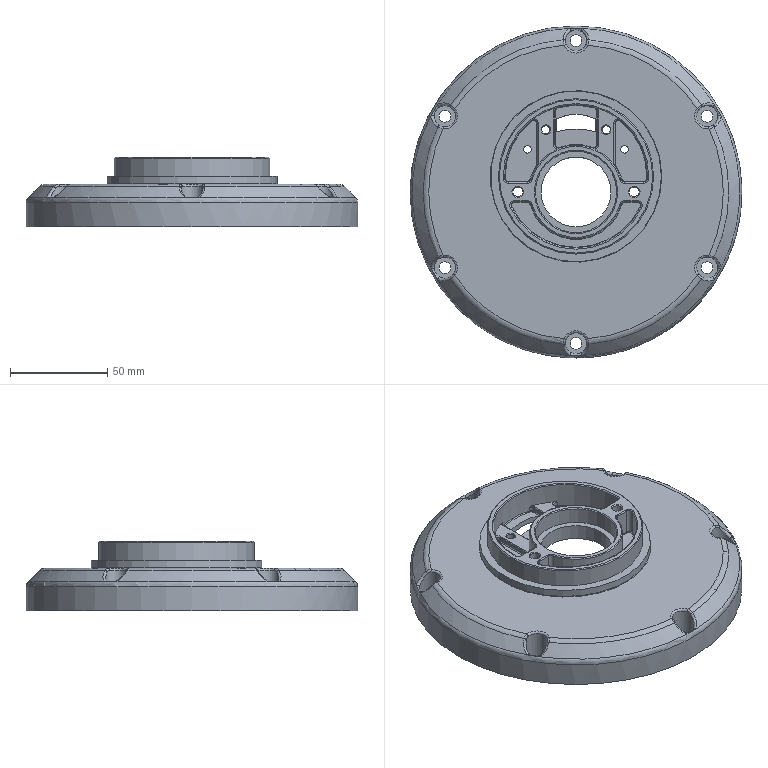Part | 1 solid | 281 faces | box 171 x 171 x 36 mm | volume 120934 mm3 | cylinder 89 | torus 76 | spline 42 | plane 28 | sphere 24 | cone 22 | commonest cylinder face diameters 4 x30 1 x20 6 x6 11 x6 17 x6 167 x6